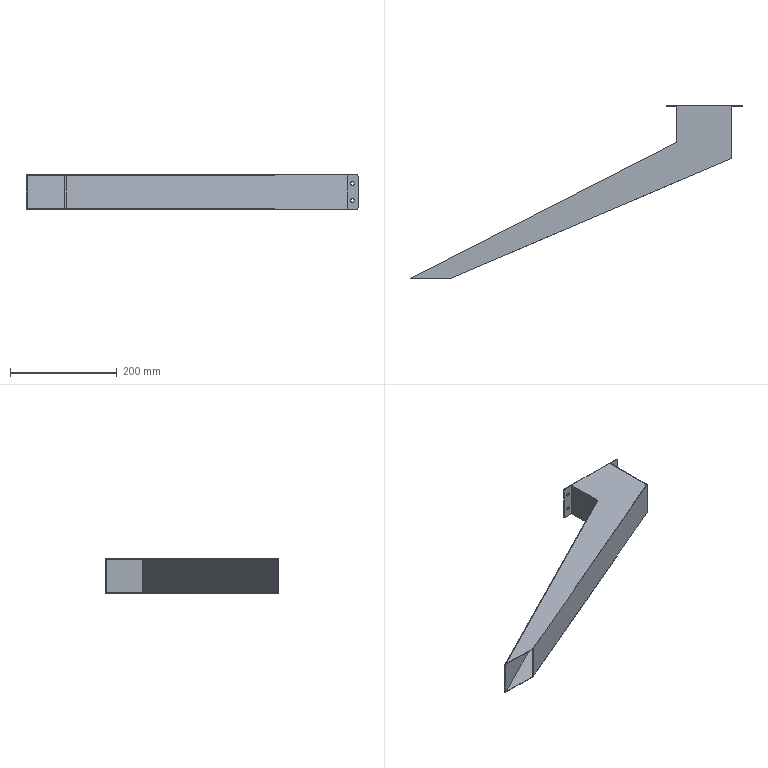Part | NX | 1 solid | 30 faces | box 622 x 324 x 65 mm | volume 159538 mm3 | plane 18 | cylinder 12 | commonest cylinder face diameters 6.4 x8 6 x4
STEP:
#1=CARTESIAN_POINT('',(1439.,-457.5,-79.28));
#2=VERTEX_POINT('',#1);
#3=CARTESIAN_POINT('',(1966.,-232.5,-79.28));
#4=VERTEX_POINT('',#3);
#5=CARTESIAN_POINT('',(1439.,-457.5,-79.28));
#6=DIRECTION('',(0.9197,0.3927,0.));
#7=VECTOR('',#6,1000.);
#8=LINE('',#5,#7);
#9=EDGE_CURVE('',#2,#4,#8,.T.);
#10=ORIENTED_EDGE('',*,*,#9,.F.);
#11=CARTESIAN_POINT('',(1439.,-457.5,-144.28));
#12=VERTEX_POINT('',#11);
#13=CARTESIAN_POINT('',(1439.,-457.5,-79.28));
#14=DIRECTION('',(0.,0.,-1.));
#15=VECTOR('',#14,1000.);
#16=LINE('',#13,#15);
#17=EDGE_CURVE('',#2,#12,#16,.T.);
#18=ORIENTED_EDGE('',*,*,#17,.T.);
#19=CARTESIAN_POINT('',(1966.,-232.5,-144.28));
#20=VERTEX_POINT('',#19);
#21=CARTESIAN_POINT('',(1439.,-457.5,-144.28));
#22=DIRECTION('',(0.9197,0.3927,0.));
#23=VECTOR('',#22,1000.);
#24=LINE('',#21,#23);
#25=EDGE_CURVE('',#12,#20,#24,.T.);
#26=ORIENTED_EDGE('',*,*,#25,.T.);
#27=CARTESIAN_POINT('',(1966.,-232.5,-79.28));
#28=DIRECTION('',(0.,0.,-1.));
#29=VECTOR('',#28,1000.);
#30=LINE('',#27,#29);
#31=EDGE_CURVE('',#4,#20,#30,.T.);
#32=ORIENTED_EDGE('',*,*,#31,.F.);
#33=EDGE_LOOP('',(#10,#18,#26,#32));
#34=FACE_BOUND('',#33,.T.);
#35=CARTESIAN_POINT('',(1439.,-457.5,-79.28));
#36=DIRECTION('',(0.3927,-0.9197,0.));
#37=DIRECTION('',(0.,0.,-1.));
#38=AXIS2_PLACEMENT_3D('',#35,#36,#37);
#39=PLANE('',#38);
#40=ADVANCED_FACE('',(#34),#39,.T.);
#41=CARTESIAN_POINT('',(1364.,-457.5,-79.28));
#42=VERTEX_POINT('',#41);
#43=CARTESIAN_POINT('',(1439.,-457.5,-79.28));
#44=DIRECTION('',(-1.,0.,0.));
#45=VECTOR('',#44,1000.);
#46=LINE('',#43,#45);
#47=EDGE_CURVE('',#2,#42,#46,.T.);
#48=ORIENTED_EDGE('',*,*,#47,.T.);
#49=CARTESIAN_POINT('',(1364.,-457.5,-144.28));
#50=VERTEX_POINT('',#49);
#51=CARTESIAN_POINT('',(1364.,-457.5,-79.28));
#52=DIRECTION('',(0.,0.,-1.));
#53=VECTOR('',#52,1000.);
#54=LINE('',#51,#53);
#55=EDGE_CURVE('',#42,#50,#54,.T.);
#56=ORIENTED_EDGE('',*,*,#55,.T.);
#57=CARTESIAN_POINT('',(1439.,-457.5,-144.28));
#58=DIRECTION('',(-1.,0.,0.));
#59=VECTOR('',#58,1000.);
#60=LINE('',#57,#59);
#61=EDGE_CURVE('',#12,#50,#60,.T.);
#62=ORIENTED_EDGE('',*,*,#61,.F.);
#63=ORIENTED_EDGE('',*,*,#17,.F.);
#64=EDGE_LOOP('',(#48,#56,#62,#63));
#65=FACE_BOUND('',#64,.T.);
#66=CARTESIAN_POINT('',(1436.453,-457.5,-143.28));
#67=VERTEX_POINT('',#66);
#68=CARTESIAN_POINT('',(1436.453,-457.5,-80.28));
#69=VERTEX_POINT('',#68);
#70=CARTESIAN_POINT('',(1436.453,-457.5,-79.28));
#71=DIRECTION('',(0.,0.,1.));
#72=VECTOR('',#71,1000.);
#73=LINE('',#70,#72);
#74=EDGE_CURVE('',#67,#69,#73,.T.);
#75=ORIENTED_EDGE('',*,*,#74,.F.);
#76=CARTESIAN_POINT('',(1366.201,-457.5,-143.28));
#77=VERTEX_POINT('',#76);
#78=CARTESIAN_POINT('',(1903.812,-457.5,-143.28));
#79=DIRECTION('',(-1.,0.,0.));
#80=VECTOR('',#79,1000.);
#81=LINE('',#78,#80);
#82=EDGE_CURVE('',#67,#77,#81,.T.);
#83=ORIENTED_EDGE('',*,*,#82,.T.);
#84=CARTESIAN_POINT('',(1366.201,-457.5,-80.28));
#85=VERTEX_POINT('',#84);
#86=CARTESIAN_POINT('',(1366.201,-457.5,-79.28));
#87=DIRECTION('',(0.,0.,-1.));
#88=VECTOR('',#87,1000.);
#89=LINE('',#86,#88);
#90=EDGE_CURVE('',#85,#77,#89,.T.);
#91=ORIENTED_EDGE('',*,*,#90,.F.);
#92=CARTESIAN_POINT('',(1903.812,-457.5,-80.28));
#93=DIRECTION('',(-1.,0.,0.));
#94=VECTOR('',#93,1000.);
#95=LINE('',#92,#94);
#96=EDGE_CURVE('',#69,#85,#95,.T.);
#97=ORIENTED_EDGE('',*,*,#96,.F.);
#98=EDGE_LOOP('',(#75,#83,#91,#97));
#99=FACE_BOUND('',#98,.T.);
#100=CARTESIAN_POINT('',(1364.,-457.5,-79.28));
#101=DIRECTION('',(0.,-1.,0.));
#102=DIRECTION('',(0.,0.,-1.));
#103=AXIS2_PLACEMENT_3D('',#100,#101,#102);
#104=PLANE('',#103);
#105=ADVANCED_FACE('',(#65,#99),#104,.T.);
#106=CARTESIAN_POINT('',(1864.,-202.5,-79.28));
#107=VERTEX_POINT('',#106);
#108=CARTESIAN_POINT('',(1364.,-457.5,-79.28));
#109=DIRECTION('',(0.8908,0.4543,0.));
#110=VECTOR('',#109,1000.);
#111=LINE('',#108,#110);
#112=EDGE_CURVE('',#42,#107,#111,.T.);
#113=ORIENTED_EDGE('',*,*,#112,.T.);
#114=CARTESIAN_POINT('',(1864.,-202.5,-144.28));
#115=VERTEX_POINT('',#114);
#116=CARTESIAN_POINT('',(1864.,-202.5,-79.28));
#117=DIRECTION('',(0.,0.,-1.));
#118=VECTOR('',#117,1000.);
#119=LINE('',#116,#118);
#120=EDGE_CURVE('',#107,#115,#119,.T.);
#121=ORIENTED_EDGE('',*,*,#120,.T.);
#122=CARTESIAN_POINT('',(1364.,-457.5,-144.28));
#123=DIRECTION('',(0.8908,0.4543,0.));
#124=VECTOR('',#123,1000.);
#125=LINE('',#122,#124);
#126=EDGE_CURVE('',#50,#115,#125,.T.);
#127=ORIENTED_EDGE('',*,*,#126,.F.);
#128=ORIENTED_EDGE('',*,*,#55,.F.);
#129=EDGE_LOOP('',(#113,#121,#127,#128));
#130=FACE_BOUND('',#129,.T.);
#131=CARTESIAN_POINT('',(1864.,-202.5,-79.28));
#132=DIRECTION('',(-0.4543,0.8908,0.));
#133=DIRECTION('',(0.,0.,1.));
#134=AXIS2_PLACEMENT_3D('',#131,#132,#133);
#135=PLANE('',#134);
#136=ADVANCED_FACE('',(#130),#135,.T.);
#137=CARTESIAN_POINT('',(1864.,-134.5,-79.28));
#138=VERTEX_POINT('',#137);
#139=CARTESIAN_POINT('',(1864.,-134.5,-144.28));
#140=VERTEX_POINT('',#139);
#141=CARTESIAN_POINT('',(1864.,-134.5,-79.28));
#142=DIRECTION('',(0.,0.,-1.));
#143=VECTOR('',#142,1000.);
#144=LINE('',#141,#143);
#145=EDGE_CURVE('',#138,#140,#144,.T.);
#146=ORIENTED_EDGE('',*,*,#145,.T.);
#147=CARTESIAN_POINT('',(1864.,-232.5,-144.28));
#148=DIRECTION('',(0.,1.,0.));
#149=VECTOR('',#148,1000.);
#150=LINE('',#147,#149);
#151=EDGE_CURVE('',#115,#140,#150,.T.);
#152=ORIENTED_EDGE('',*,*,#151,.F.);
#153=ORIENTED_EDGE('',*,*,#120,.F.);
#154=CARTESIAN_POINT('',(1864.,-232.5,-79.28));
#155=DIRECTION('',(0.,1.,0.));
#156=VECTOR('',#155,1000.);
#157=LINE('',#154,#156);
#158=EDGE_CURVE('',#107,#138,#157,.T.);
#159=ORIENTED_EDGE('',*,*,#158,.T.);
#160=EDGE_LOOP('',(#146,#152,#153,#159));
#161=FACE_BOUND('',#160,.T.);
#162=CARTESIAN_POINT('',(1864.,-133.5,-79.28));
#163=DIRECTION('',(-1.,0.,0.));
#164=DIRECTION('',(0.,0.,1.));
#165=AXIS2_PLACEMENT_3D('',#162,#163,#164);
#166=PLANE('',#165);
#167=ADVANCED_FACE('',(#161),#166,.T.);
#168=CARTESIAN_POINT('',(1966.,-134.5,-79.28));
#169=VERTEX_POINT('',#168);
#170=CARTESIAN_POINT('',(1966.,-133.5,-79.28));
#171=DIRECTION('',(0.,-1.,0.));
#172=VECTOR('',#171,1000.);
#173=LINE('',#170,#172);
#174=EDGE_CURVE('',#169,#4,#173,.T.);
#175=ORIENTED_EDGE('',*,*,#174,.T.);
#176=ORIENTED_EDGE('',*,*,#31,.T.);
#177=CARTESIAN_POINT('',(1966.,-134.5,-144.28));
#178=VERTEX_POINT('',#177);
#179=CARTESIAN_POINT('',(1966.,-133.5,-144.28));
#180=DIRECTION('',(0.,-1.,0.));
#181=VECTOR('',#180,1000.);
#182=LINE('',#179,#181);
#183=EDGE_CURVE('',#178,#20,#182,.T.);
#184=ORIENTED_EDGE('',*,*,#183,.F.);
#185=CARTESIAN_POINT('',(1966.,-134.5,-79.28));
#186=DIRECTION('',(0.,0.,1.));
#187=VECTOR('',#186,1000.);
#188=LINE('',#185,#187);
#189=EDGE_CURVE('',#178,#169,#188,.T.);
#190=ORIENTED_EDGE('',*,*,#189,.T.);
#191=EDGE_LOOP('',(#175,#176,#184,#190));
#192=FACE_BOUND('',#191,.T.);
#193=CARTESIAN_POINT('',(1966.,-232.5,-79.28));
#194=DIRECTION('',(1.,0.,0.));
#195=DIRECTION('',(0.,1.,0.));
#196=AXIS2_PLACEMENT_3D('',#193,#194,#195);
#197=PLANE('',#196);
#198=ADVANCED_FACE('',(#192),#197,.T.);
#199=CARTESIAN_POINT('',(1965.,-133.5,-80.28));
#200=VERTEX_POINT('',#199);
#201=CARTESIAN_POINT('',(1965.,-231.84,-80.28));
#202=VERTEX_POINT('',#201);
#203=CARTESIAN_POINT('',(1965.,-133.5,-80.28));
#204=DIRECTION('',(0.,-1.,0.));
#205=VECTOR('',#204,1000.);
#206=LINE('',#203,#205);
#207=EDGE_CURVE('',#200,#202,#206,.T.);
#208=ORIENTED_EDGE('',*,*,#207,.T.);
#209=CARTESIAN_POINT('',(1903.812,-257.964,-80.28));
#210=DIRECTION('',(0.9197,0.3927,0.));
#211=VECTOR('',#210,1000.);
#212=LINE('',#209,#211);
#213=EDGE_CURVE('',#69,#202,#212,.T.);
#214=ORIENTED_EDGE('',*,*,#213,.F.);
#215=ORIENTED_EDGE('',*,*,#96,.T.);
#216=CARTESIAN_POINT('',(1865.,-203.113,-80.28));
#217=VERTEX_POINT('',#216);
#218=CARTESIAN_POINT('',(1903.812,-183.319,-80.28));
#219=DIRECTION('',(0.8908,0.4543,0.));
#220=VECTOR('',#219,1000.);
#221=LINE('',#218,#220);
#222=EDGE_CURVE('',#85,#217,#221,.T.);
#223=ORIENTED_EDGE('',*,*,#222,.T.);
#224=CARTESIAN_POINT('',(1865.,-133.5,-80.28));
#225=VERTEX_POINT('',#224);
#226=CARTESIAN_POINT('',(1865.,-24.838,-80.28));
#227=DIRECTION('',(0.,-1.,0.));
#228=VECTOR('',#227,1000.);
#229=LINE('',#226,#228);
#230=EDGE_CURVE('',#225,#217,#229,.T.);
#231=ORIENTED_EDGE('',*,*,#230,.F.);
#232=CARTESIAN_POINT('',(1903.812,-133.5,-80.28));
#233=DIRECTION('',(1.,0.,0.));
#234=VECTOR('',#233,1000.);
#235=LINE('',#232,#234);
#236=EDGE_CURVE('',#225,#200,#235,.T.);
#237=ORIENTED_EDGE('',*,*,#236,.T.);
#238=EDGE_LOOP('',(#208,#214,#215,#223,#231,#237));
#239=FACE_BOUND('',#238,.T.);
#240=CARTESIAN_POINT('',(1903.812,-24.838,-80.28));
#241=DIRECTION('',(0.,0.,1.));
#242=DIRECTION('',(1.,0.,0.));
#243=AXIS2_PLACEMENT_3D('',#240,#241,#242);
#244=PLANE('',#243);
#245=ADVANCED_FACE('',(#239),#244,.F.);
#246=CARTESIAN_POINT('',(1965.,-231.84,-143.28));
#247=VERTEX_POINT('',#246);
#248=CARTESIAN_POINT('',(1965.,-231.84,-79.28));
#249=DIRECTION('',(0.,0.,-1.));
#250=VECTOR('',#249,1000.);
#251=LINE('',#248,#250);
#252=EDGE_CURVE('',#202,#247,#251,.T.);
#253=ORIENTED_EDGE('',*,*,#252,.T.);
#254=CARTESIAN_POINT('',(1903.812,-257.964,-143.28));
#255=DIRECTION('',(0.9197,0.3927,0.));
#256=VECTOR('',#255,1000.);
#257=LINE('',#254,#256);
#258=EDGE_CURVE('',#67,#247,#257,.T.);
#259=ORIENTED_EDGE('',*,*,#258,.F.);
#260=ORIENTED_EDGE('',*,*,#74,.T.);
#261=ORIENTED_EDGE('',*,*,#213,.T.);
#262=EDGE_LOOP('',(#253,#259,#260,#261));
#263=FACE_BOUND('',#262,.T.);
#264=CARTESIAN_POINT('',(1438.607,-456.58,-79.28));
#265=DIRECTION('',(0.3927,-0.9197,0.));
#266=DIRECTION('',(0.,0.,-1.));
#267=AXIS2_PLACEMENT_3D('',#264,#265,#266);
#268=PLANE('',#267);
#269=ADVANCED_FACE('',(#263),#268,.F.);
#270=CARTESIAN_POINT('',(1965.,-133.5,-143.28));
#271=VERTEX_POINT('',#270);
#272=CARTESIAN_POINT('',(1965.,-24.838,-143.28));
#273=DIRECTION('',(0.,-1.,0.));
#274=VECTOR('',#273,1000.);
#275=LINE('',#272,#274);
#276=EDGE_CURVE('',#271,#247,#275,.T.);
#277=ORIENTED_EDGE('',*,*,#276,.T.);
#278=ORIENTED_EDGE('',*,*,#252,.F.);
#279=ORIENTED_EDGE('',*,*,#207,.F.);
#280=CARTESIAN_POINT('',(1965.,-133.5,-79.28));
#281=DIRECTION('',(0.,0.,-1.));
#282=VECTOR('',#281,1000.);
#283=LINE('',#280,#282);
#284=EDGE_CURVE('',#200,#271,#283,.T.);
#285=ORIENTED_EDGE('',*,*,#284,.T.);
#286=EDGE_LOOP('',(#277,#278,#279,#285));
#287=FACE_BOUND('',#286,.T.);
#288=CARTESIAN_POINT('',(1965.,-232.5,-79.28));
#289=DIRECTION('',(1.,0.,0.));
#290=DIRECTION('',(0.,1.,0.));
#291=AXIS2_PLACEMENT_3D('',#288,#289,#290);
#292=PLANE('',#291);
#293=ADVANCED_FACE('',(#287),#292,.F.);
#294=CARTESIAN_POINT('',(1865.,-203.113,-143.28));
#295=VERTEX_POINT('',#294);
#296=CARTESIAN_POINT('',(1865.,-133.5,-143.28));
#297=VERTEX_POINT('',#296);
#298=CARTESIAN_POINT('',(1865.,-24.838,-143.28));
#299=DIRECTION('',(0.,1.,0.));
#300=VECTOR('',#299,1000.);
#301=LINE('',#298,#300);
#302=EDGE_CURVE('',#295,#297,#301,.T.);
#303=ORIENTED_EDGE('',*,*,#302,.F.);
#304=CARTESIAN_POINT('',(1903.812,-183.319,-143.28));
#305=DIRECTION('',(0.8908,0.4543,0.));
#306=VECTOR('',#305,1000.);
#307=LINE('',#304,#306);
#308=EDGE_CURVE('',#77,#295,#307,.T.);
#309=ORIENTED_EDGE('',*,*,#308,.F.);
#310=ORIENTED_EDGE('',*,*,#82,.F.);
#311=ORIENTED_EDGE('',*,*,#258,.T.);
#312=ORIENTED_EDGE('',*,*,#276,.F.);
#313=CARTESIAN_POINT('',(1903.812,-133.5,-143.28));
#314=DIRECTION('',(-1.,0.,0.));
#315=VECTOR('',#314,1000.);
#316=LINE('',#313,#315);
#317=EDGE_CURVE('',#271,#297,#316,.T.);
#318=ORIENTED_EDGE('',*,*,#317,.T.);
#319=EDGE_LOOP('',(#303,#309,#310,#311,#312,#318));
#320=FACE_BOUND('',#319,.T.);
#321=CARTESIAN_POINT('',(1903.812,-24.838,-143.28));
#322=DIRECTION('',(0.,0.,1.));
#323=DIRECTION('',(1.,0.,0.));
#324=AXIS2_PLACEMENT_3D('',#321,#322,#323);
#325=PLANE('',#324);
#326=ADVANCED_FACE('',(#320),#325,.T.);
#327=ORIENTED_EDGE('',*,*,#230,.T.);
#328=CARTESIAN_POINT('',(1865.,-203.113,-79.28));
#329=DIRECTION('',(0.,0.,-1.));
#330=VECTOR('',#329,1000.);
#331=LINE('',#328,#330);
#332=EDGE_CURVE('',#217,#295,#331,.T.);
#333=ORIENTED_EDGE('',*,*,#332,.T.);
#334=ORIENTED_EDGE('',*,*,#302,.T.);
#335=CARTESIAN_POINT('',(1865.,-133.5,-79.28));
#336=DIRECTION('',(0.,0.,1.));
#337=VECTOR('',#336,1000.);
#338=LINE('',#335,#337);
#339=EDGE_CURVE('',#297,#225,#338,.T.);
#340=ORIENTED_EDGE('',*,*,#339,.T.);
#341=EDGE_LOOP('',(#327,#333,#334,#340));
#342=FACE_BOUND('',#341,.T.);
#343=CARTESIAN_POINT('',(1865.,-133.5,-79.28));
#344=DIRECTION('',(-1.,0.,0.));
#345=DIRECTION('',(0.,0.,1.));
#346=AXIS2_PLACEMENT_3D('',#343,#344,#345);
#347=PLANE('',#346);
#348=ADVANCED_FACE('',(#342),#347,.F.);
#349=ORIENTED_EDGE('',*,*,#90,.T.);
#350=ORIENTED_EDGE('',*,*,#308,.T.);
#351=ORIENTED_EDGE('',*,*,#332,.F.);
#352=ORIENTED_EDGE('',*,*,#222,.F.);
#353=EDGE_LOOP('',(#349,#350,#351,#352));
#354=FACE_BOUND('',#353,.T.);
#355=CARTESIAN_POINT('',(1864.454,-203.391,-79.28));
#356=DIRECTION('',(-0.4543,0.8908,0.));
#357=DIRECTION('',(0.,0.,1.));
#358=AXIS2_PLACEMENT_3D('',#355,#356,#357);
#359=PLANE('',#358);
#360=ADVANCED_FACE('',(#354),#359,.F.);
#361=ORIENTED_EDGE('',*,*,#126,.T.);
#362=ORIENTED_EDGE('',*,*,#151,.T.);
#363=CARTESIAN_POINT('',(1847.,-134.5,-144.28));
#364=VERTEX_POINT('',#363);
#365=CARTESIAN_POINT('',(1915.,-134.5,-144.28));
#366=DIRECTION('',(1.,0.,0.));
#367=VECTOR('',#366,1000.);
#368=LINE('',#365,#367);
#369=EDGE_CURVE('',#364,#140,#368,.T.);
#370=ORIENTED_EDGE('',*,*,#369,.F.);
#371=CARTESIAN_POINT('',(1847.,-133.5,-144.28));
#372=VERTEX_POINT('',#371);
#373=CARTESIAN_POINT('',(1847.,-133.5,-144.28));
#374=DIRECTION('',(0.,-1.,0.));
#375=VECTOR('',#374,1000.);
#376=LINE('',#373,#375);
#377=EDGE_CURVE('',#372,#364,#376,.T.);
#378=ORIENTED_EDGE('',*,*,#377,.F.);
#379=CARTESIAN_POINT('',(1983.,-133.5,-144.28));
#380=VERTEX_POINT('',#379);
#381=CARTESIAN_POINT('',(1915.,-133.5,-144.28));
#382=DIRECTION('',(1.,0.,0.));
#383=VECTOR('',#382,1000.);
#384=LINE('',#381,#383);
#385=EDGE_CURVE('',#372,#380,#384,.T.);
#386=ORIENTED_EDGE('',*,*,#385,.T.);
#387=CARTESIAN_POINT('',(1983.,-134.5,-144.28));
#388=VERTEX_POINT('',#387);
#389=CARTESIAN_POINT('',(1983.,-133.5,-144.28));
#390=DIRECTION('',(0.,-1.,0.));
#391=VECTOR('',#390,1000.);
#392=LINE('',#389,#391);
#393=EDGE_CURVE('',#380,#388,#392,.T.);
#394=ORIENTED_EDGE('',*,*,#393,.T.);
#395=CARTESIAN_POINT('',(1915.,-134.5,-144.28));
#396=DIRECTION('',(1.,0.,0.));
#397=VECTOR('',#396,1000.);
#398=LINE('',#395,#397);
#399=EDGE_CURVE('',#178,#388,#398,.T.);
#400=ORIENTED_EDGE('',*,*,#399,.F.);
#401=ORIENTED_EDGE('',*,*,#183,.T.);
#402=ORIENTED_EDGE('',*,*,#25,.F.);
#403=ORIENTED_EDGE('',*,*,#61,.T.);
#404=EDGE_LOOP('',(#361,#362,#370,#378,#386,#394,#400,#401,#402,#403));
#405=FACE_BOUND('',#404,.T.);
#406=CARTESIAN_POINT('',(1903.812,-24.838,-144.28));
#407=DIRECTION('',(0.,0.,1.));
#408=DIRECTION('',(1.,0.,0.));
#409=AXIS2_PLACEMENT_3D('',#406,#407,#408);
#410=PLANE('',#409);
#411=ADVANCED_FACE('',(#405),#410,.F.);
#412=CARTESIAN_POINT('',(1986.,-133.5,-141.28));
#413=VERTEX_POINT('',#412);
#414=CARTESIAN_POINT('',(1983.,-133.5,-141.28));
#415=DIRECTION('',(0.,1.,0.));
#416=DIRECTION('',(1.,0.,0.));
#417=AXIS2_PLACEMENT_3D('',#414,#415,#416);
#418=CIRCLE('',#417,3.);
#419=EDGE_CURVE('',#413,#380,#418,.T.);
#420=ORIENTED_EDGE('',*,*,#419,.F.);
#421=CARTESIAN_POINT('',(1986.,-134.5,-141.28));
#422=VERTEX_POINT('',#421);
#423=CARTESIAN_POINT('',(1986.,-133.5,-141.28));
#424=DIRECTION('',(0.,-1.,0.));
#425=VECTOR('',#424,1000.);
#426=LINE('',#423,#425);
#427=EDGE_CURVE('',#413,#422,#426,.T.);
#428=ORIENTED_EDGE('',*,*,#427,.T.);
#429=CARTESIAN_POINT('',(1983.,-134.5,-141.28));
#430=DIRECTION('',(0.,1.,0.));
#431=DIRECTION('',(1.,0.,0.));
#432=AXIS2_PLACEMENT_3D('',#429,#430,#431);
#433=CIRCLE('',#432,3.);
#434=EDGE_CURVE('',#422,#388,#433,.T.);
#435=ORIENTED_EDGE('',*,*,#434,.T.);
#436=ORIENTED_EDGE('',*,*,#393,.F.);
#437=EDGE_LOOP('',(#420,#428,#435,#436));
#438=FACE_BOUND('',#437,.T.);
#439=CARTESIAN_POINT('',(1983.,-133.5,-141.28));
#440=DIRECTION('',(0.,1.,0.));
#441=DIRECTION('',(1.,0.,0.));
#442=AXIS2_PLACEMENT_3D('',#439,#440,#441);
#443=CYLINDRICAL_SURFACE('',#442,3.);
#444=ADVANCED_FACE('',(#438),#443,.T.);
#445=CARTESIAN_POINT('',(1978.7,-134.5,-127.53));
#446=VERTEX_POINT('',#445);
#447=CARTESIAN_POINT('',(1972.3,-134.5,-127.53));
#448=VERTEX_POINT('',#447);
#449=CARTESIAN_POINT('',(1975.5,-134.5,-127.53));
#450=DIRECTION('',(0.,-1.,0.));
#451=DIRECTION('',(-1.,0.,0.));
#452=AXIS2_PLACEMENT_3D('',#449,#450,#451);
#453=CIRCLE('',#452,3.2);
#454=EDGE_CURVE('',#446,#448,#453,.T.);
#455=ORIENTED_EDGE('',*,*,#454,.T.);
#456=CARTESIAN_POINT('',(1972.3,-133.5,-127.53));
#457=VERTEX_POINT('',#456);
#458=CARTESIAN_POINT('',(1972.3,-133.5,-127.53));
#459=DIRECTION('',(0.,-1.,0.));
#460=VECTOR('',#459,1000.);
#461=LINE('',#458,#460);
#462=EDGE_CURVE('',#448,#457,#461,.F.);
#463=ORIENTED_EDGE('',*,*,#462,.T.);
#464=CARTESIAN_POINT('',(1978.7,-133.5,-127.53));
#465=VERTEX_POINT('',#464);
#466=CARTESIAN_POINT('',(1975.5,-133.5,-127.53));
#467=DIRECTION('',(0.,-1.,0.));
#468=DIRECTION('',(-1.,0.,0.));
#469=AXIS2_PLACEMENT_3D('',#466,#467,#468);
#470=CIRCLE('',#469,3.2);
#471=EDGE_CURVE('',#465,#457,#470,.T.);
#472=ORIENTED_EDGE('',*,*,#471,.F.);
#473=CARTESIAN_POINT('',(1978.7,-133.5,-127.53));
#474=DIRECTION('',(0.,-1.,0.));
#475=VECTOR('',#474,1000.);
#476=LINE('',#473,#475);
#477=EDGE_CURVE('',#446,#465,#476,.F.);
#478=ORIENTED_EDGE('',*,*,#477,.F.);
#479=EDGE_LOOP('',(#455,#463,#472,#478));
#480=FACE_BOUND('',#479,.T.);
#481=CARTESIAN_POINT('',(1975.5,-133.5,-127.53));
#482=DIRECTION('',(0.,-1.,0.));
#483=DIRECTION('',(-1.,0.,0.));
#484=AXIS2_PLACEMENT_3D('',#481,#482,#483);
#485=CYLINDRICAL_SURFACE('',#484,3.2);
#486=ADVANCED_FACE('',(#480),#485,.F.);
#487=CARTESIAN_POINT('',(1978.7,-134.5,-96.03));
#488=VERTEX_POINT('',#487);
#489=CARTESIAN_POINT('',(1972.3,-134.5,-96.03));
#490=VERTEX_POINT('',#489);
#491=CARTESIAN_POINT('',(1975.5,-134.5,-96.03));
#492=DIRECTION('',(0.,-1.,0.));
#493=DIRECTION('',(-1.,0.,0.));
#494=AXIS2_PLACEMENT_3D('',#491,#492,#493);
#495=CIRCLE('',#494,3.2);
#496=EDGE_CURVE('',#488,#490,#495,.T.);
#497=ORIENTED_EDGE('',*,*,#496,.T.);
#498=CARTESIAN_POINT('',(1972.3,-133.5,-96.03));
#499=VERTEX_POINT('',#498);
#500=CARTESIAN_POINT('',(1972.3,-133.5,-96.03));
#501=DIRECTION('',(0.,-1.,0.));
#502=VECTOR('',#501,1000.);
#503=LINE('',#500,#502);
#504=EDGE_CURVE('',#490,#499,#503,.F.);
#505=ORIENTED_EDGE('',*,*,#504,.T.);
#506=CARTESIAN_POINT('',(1978.7,-133.5,-96.03));
#507=VERTEX_POINT('',#506);
#508=CARTESIAN_POINT('',(1975.5,-133.5,-96.03));
#509=DIRECTION('',(0.,-1.,0.));
#510=DIRECTION('',(-1.,0.,0.));
#511=AXIS2_PLACEMENT_3D('',#508,#509,#510);
#512=CIRCLE('',#511,3.2);
#513=EDGE_CURVE('',#507,#499,#512,.T.);
#514=ORIENTED_EDGE('',*,*,#513,.F.);
#515=CARTESIAN_POINT('',(1978.7,-133.5,-96.03));
#516=DIRECTION('',(0.,-1.,0.));
#517=VECTOR('',#516,1000.);
#518=LINE('',#515,#517);
#519=EDGE_CURVE('',#488,#507,#518,.F.);
#520=ORIENTED_EDGE('',*,*,#519,.F.);
#521=EDGE_LOOP('',(#497,#505,#514,#520));
#522=FACE_BOUND('',#521,.T.);
#523=CARTESIAN_POINT('',(1975.5,-133.5,-96.03));
#524=DIRECTION('',(0.,-1.,0.));
#525=DIRECTION('',(-1.,0.,0.));
#526=AXIS2_PLACEMENT_3D('',#523,#524,#525);
#527=CYLINDRICAL_SURFACE('',#526,3.2);
#528=ADVANCED_FACE('',(#522),#527,.F.);
#529=ORIENTED_EDGE('',*,*,#399,.T.);
#530=ORIENTED_EDGE('',*,*,#434,.F.);
#531=CARTESIAN_POINT('',(1986.,-134.5,-82.28));
#532=VERTEX_POINT('',#531);
#533=CARTESIAN_POINT('',(1986.,-134.5,-130.28));
#534=DIRECTION('',(0.,0.,-1.));
#535=VECTOR('',#534,1000.);
#536=LINE('',#533,#535);
#537=EDGE_CURVE('',#532,#422,#536,.T.);
#538=ORIENTED_EDGE('',*,*,#537,.F.);
#539=CARTESIAN_POINT('',(1983.,-134.5,-79.28));
#540=VERTEX_POINT('',#539);
#541=CARTESIAN_POINT('',(1983.,-134.5,-82.28));
#542=DIRECTION('',(0.,1.,0.));
#543=DIRECTION('',(1.,0.,0.));
#544=AXIS2_PLACEMENT_3D('',#541,#542,#543);
#545=CIRCLE('',#544,3.);
#546=EDGE_CURVE('',#540,#532,#545,.T.);
#547=ORIENTED_EDGE('',*,*,#546,.F.);
#548=CARTESIAN_POINT('',(1915.,-134.5,-79.28));
#549=DIRECTION('',(1.,0.,0.));
#550=VECTOR('',#549,1000.);
#551=LINE('',#548,#550);
#552=EDGE_CURVE('',#169,#540,#551,.T.);
#553=ORIENTED_EDGE('',*,*,#552,.F.);
#554=ORIENTED_EDGE('',*,*,#189,.F.);
#555=EDGE_LOOP('',(#529,#530,#538,#547,#553,#554));
#556=FACE_BOUND('',#555,.T.);
#557=ORIENTED_EDGE('',*,*,#454,.F.);
#558=CARTESIAN_POINT('',(1975.5,-134.5,-127.53));
#559=DIRECTION('',(0.,-1.,0.));
#560=DIRECTION('',(-1.,0.,0.));
#561=AXIS2_PLACEMENT_3D('',#558,#559,#560);
#562=CIRCLE('',#561,3.2);
#563=EDGE_CURVE('',#448,#446,#562,.T.);
#564=ORIENTED_EDGE('',*,*,#563,.F.);
#565=EDGE_LOOP('',(#557,#564));
#566=FACE_BOUND('',#565,.T.);
#567=ORIENTED_EDGE('',*,*,#496,.F.);
#568=CARTESIAN_POINT('',(1975.5,-134.5,-96.03));
#569=DIRECTION('',(0.,-1.,0.));
#570=DIRECTION('',(-1.,0.,0.));
#571=AXIS2_PLACEMENT_3D('',#568,#569,#570);
#572=CIRCLE('',#571,3.2);
#573=EDGE_CURVE('',#490,#488,#572,.T.);
#574=ORIENTED_EDGE('',*,*,#573,.F.);
#575=EDGE_LOOP('',(#567,#574));
#576=FACE_BOUND('',#575,.T.);
#577=CARTESIAN_POINT('',(1876.658,-134.5,-112.212));
#578=DIRECTION('',(0.,1.,0.));
#579=DIRECTION('',(1.,0.,0.));
#580=AXIS2_PLACEMENT_3D('',#577,#578,#579);
#581=PLANE('',#580);
#582=ADVANCED_FACE('',(#556,#566,#576),#581,.F.);
#583=CARTESIAN_POINT('',(1983.,-133.5,-79.28));
#584=VERTEX_POINT('',#583);
#585=CARTESIAN_POINT('',(1986.,-133.5,-82.28));
#586=VERTEX_POINT('',#585);
#587=CARTESIAN_POINT('',(1983.,-133.5,-82.28));
#588=DIRECTION('',(0.,1.,0.));
#589=DIRECTION('',(1.,0.,0.));
#590=AXIS2_PLACEMENT_3D('',#587,#588,#589);
#591=CIRCLE('',#590,3.);
#592=EDGE_CURVE('',#584,#586,#591,.T.);
#593=ORIENTED_EDGE('',*,*,#592,.F.);
#594=CARTESIAN_POINT('',(1983.,-133.5,-79.28));
#595=DIRECTION('',(0.,-1.,0.));
#596=VECTOR('',#595,1000.);
#597=LINE('',#594,#596);
#598=EDGE_CURVE('',#584,#540,#597,.T.);
#599=ORIENTED_EDGE('',*,*,#598,.T.);
#600=ORIENTED_EDGE('',*,*,#546,.T.);
#601=CARTESIAN_POINT('',(1986.,-133.5,-82.28));
#602=DIRECTION('',(0.,-1.,0.));
#603=VECTOR('',#602,1000.);
#604=LINE('',#601,#603);
#605=EDGE_CURVE('',#586,#532,#604,.T.);
#606=ORIENTED_EDGE('',*,*,#605,.F.);
#607=EDGE_LOOP('',(#593,#599,#600,#606));
#608=FACE_BOUND('',#607,.T.);
#609=CARTESIAN_POINT('',(1983.,-133.5,-82.28));
#610=DIRECTION('',(0.,1.,0.));
#611=DIRECTION('',(1.,0.,0.));
#612=AXIS2_PLACEMENT_3D('',#609,#610,#611);
#613=CYLINDRICAL_SURFACE('',#612,3.);
#614=ADVANCED_FACE('',(#608),#613,.T.);
#615=CARTESIAN_POINT('',(1986.,-133.5,-130.28));
#616=DIRECTION('',(0.,0.,-1.));
#617=VECTOR('',#616,1000.);
#618=LINE('',#615,#617);
#619=EDGE_CURVE('',#586,#413,#618,.T.);
#620=ORIENTED_EDGE('',*,*,#619,.F.);
#621=ORIENTED_EDGE('',*,*,#605,.T.);
#622=ORIENTED_EDGE('',*,*,#537,.T.);
#623=ORIENTED_EDGE('',*,*,#427,.F.);
#624=EDGE_LOOP('',(#620,#621,#622,#623));
#625=FACE_BOUND('',#624,.T.);
#626=CARTESIAN_POINT('',(1986.,-133.5,-82.28));
#627=DIRECTION('',(1.,0.,0.));
#628=DIRECTION('',(0.,1.,0.));
#629=AXIS2_PLACEMENT_3D('',#626,#627,#628);
#630=PLANE('',#629);
#631=ADVANCED_FACE('',(#625),#630,.T.);
#632=ORIENTED_EDGE('',*,*,#462,.F.);
#633=ORIENTED_EDGE('',*,*,#563,.T.);
#634=ORIENTED_EDGE('',*,*,#477,.T.);
#635=CARTESIAN_POINT('',(1975.5,-133.5,-127.53));
#636=DIRECTION('',(0.,-1.,0.));
#637=DIRECTION('',(-1.,0.,0.));
#638=AXIS2_PLACEMENT_3D('',#635,#636,#637);
#639=CIRCLE('',#638,3.2);
#640=EDGE_CURVE('',#457,#465,#639,.T.);
#641=ORIENTED_EDGE('',*,*,#640,.F.);
#642=EDGE_LOOP('',(#632,#633,#634,#641));
#643=FACE_BOUND('',#642,.T.);
#644=CARTESIAN_POINT('',(1975.5,-133.5,-127.53));
#645=DIRECTION('',(0.,-1.,0.));
#646=DIRECTION('',(-1.,0.,0.));
#647=AXIS2_PLACEMENT_3D('',#644,#645,#646);
#648=CYLINDRICAL_SURFACE('',#647,3.2);
#649=ADVANCED_FACE('',(#643),#648,.F.);
#650=ORIENTED_EDGE('',*,*,#504,.F.);
#651=ORIENTED_EDGE('',*,*,#573,.T.);
#652=ORIENTED_EDGE('',*,*,#519,.T.);
#653=CARTESIAN_POINT('',(1975.5,-133.5,-96.03));
#654=DIRECTION('',(0.,-1.,0.));
#655=DIRECTION('',(-1.,0.,0.));
#656=AXIS2_PLACEMENT_3D('',#653,#654,#655);
#657=CIRCLE('',#656,3.2);
#658=EDGE_CURVE('',#499,#507,#657,.T.);
#659=ORIENTED_EDGE('',*,*,#658,.F.);
#660=EDGE_LOOP('',(#650,#651,#652,#659));
#661=FACE_BOUND('',#660,.T.);
#662=CARTESIAN_POINT('',(1975.5,-133.5,-96.03));
#663=DIRECTION('',(0.,-1.,0.));
#664=DIRECTION('',(-1.,0.,0.));
#665=AXIS2_PLACEMENT_3D('',#662,#663,#664);
#666=CYLINDRICAL_SURFACE('',#665,3.2);
#667=ADVANCED_FACE('',(#661),#666,.F.);
#668=CARTESIAN_POINT('',(1857.7,-134.5,-96.03));
#669=VERTEX_POINT('',#668);
#670=CARTESIAN_POINT('',(1851.3,-134.5,-96.03));
#671=VERTEX_POINT('',#670);
#672=CARTESIAN_POINT('',(1854.5,-134.5,-96.03));
#673=DIRECTION('',(0.,-1.,0.));
#674=DIRECTION('',(-1.,0.,0.));
#675=AXIS2_PLACEMENT_3D('',#672,#673,#674);
#676=CIRCLE('',#675,3.2);
#677=EDGE_CURVE('',#669,#671,#676,.T.);
#678=ORIENTED_EDGE('',*,*,#677,.T.);
#679=CARTESIAN_POINT('',(1851.3,-133.5,-96.03));
#680=VERTEX_POINT('',#679);
#681=CARTESIAN_POINT('',(1851.3,-133.5,-96.03));
#682=DIRECTION('',(0.,-1.,0.));
#683=VECTOR('',#682,1000.);
#684=LINE('',#681,#683);
#685=EDGE_CURVE('',#671,#680,#684,.F.);
#686=ORIENTED_EDGE('',*,*,#685,.T.);
#687=CARTESIAN_POINT('',(1857.7,-133.5,-96.03));
#688=VERTEX_POINT('',#687);
#689=CARTESIAN_POINT('',(1854.5,-133.5,-96.03));
#690=DIRECTION('',(0.,-1.,0.));
#691=DIRECTION('',(-1.,0.,0.));
#692=AXIS2_PLACEMENT_3D('',#689,#690,#691);
#693=CIRCLE('',#692,3.2);
#694=EDGE_CURVE('',#688,#680,#693,.T.);
#695=ORIENTED_EDGE('',*,*,#694,.F.);
#696=CARTESIAN_POINT('',(1857.7,-133.5,-96.03));
#697=DIRECTION('',(0.,-1.,0.));
#698=VECTOR('',#697,1000.);
#699=LINE('',#696,#698);
#700=EDGE_CURVE('',#669,#688,#699,.F.);
#701=ORIENTED_EDGE('',*,*,#700,.F.);
#702=EDGE_LOOP('',(#678,#686,#695,#701));
#703=FACE_BOUND('',#702,.T.);
#704=CARTESIAN_POINT('',(1854.5,-133.5,-96.03));
#705=DIRECTION('',(0.,-1.,0.));
#706=DIRECTION('',(-1.,0.,0.));
#707=AXIS2_PLACEMENT_3D('',#704,#705,#706);
#708=CYLINDRICAL_SURFACE('',#707,3.2);
#709=ADVANCED_FACE('',(#703),#708,.F.);
#710=ORIENTED_EDGE('',*,*,#552,.T.);
#711=ORIENTED_EDGE('',*,*,#598,.F.);
#712=CARTESIAN_POINT('',(1847.,-133.5,-79.28));
#713=VERTEX_POINT('',#712);
#714=CARTESIAN_POINT('',(1915.,-133.5,-79.28));
#715=DIRECTION('',(1.,0.,0.));
#716=VECTOR('',#715,1000.);
#717=LINE('',#714,#716);
#718=EDGE_CURVE('',#713,#584,#717,.T.);
#719=ORIENTED_EDGE('',*,*,#718,.F.);
#720=CARTESIAN_POINT('',(1847.,-134.5,-79.28));
#721=VERTEX_POINT('',#720);
#722=CARTESIAN_POINT('',(1847.,-133.5,-79.28));
#723=DIRECTION('',(0.,-1.,0.));
#724=VECTOR('',#723,1000.);
#725=LINE('',#722,#724);
#726=EDGE_CURVE('',#713,#721,#725,.T.);
#727=ORIENTED_EDGE('',*,*,#726,.T.);
#728=CARTESIAN_POINT('',(1915.,-134.5,-79.28));
#729=DIRECTION('',(1.,0.,0.));
#730=VECTOR('',#729,1000.);
#731=LINE('',#728,#730);
#732=EDGE_CURVE('',#721,#138,#731,.T.);
#733=ORIENTED_EDGE('',*,*,#732,.T.);
#734=ORIENTED_EDGE('',*,*,#158,.F.);
#735=ORIENTED_EDGE('',*,*,#112,.F.);
#736=ORIENTED_EDGE('',*,*,#47,.F.);
#737=ORIENTED_EDGE('',*,*,#9,.T.);
#738=ORIENTED_EDGE('',*,*,#174,.F.);
#739=EDGE_LOOP('',(#710,#711,#719,#727,#733,#734,#735,#736,#737,#738));
#740=FACE_BOUND('',#739,.T.);
#741=CARTESIAN_POINT('',(1903.812,-24.838,-79.28));
#742=DIRECTION('',(0.,0.,1.));
#743=DIRECTION('',(1.,0.,0.));
#744=AXIS2_PLACEMENT_3D('',#741,#742,#743);
#745=PLANE('',#744);
#746=ADVANCED_FACE('',(#740),#745,.T.);
#747=CARTESIAN_POINT('',(1844.,-133.5,-82.28));
#748=VERTEX_POINT('',#747);
#749=CARTESIAN_POINT('',(1847.,-133.5,-82.28));
#750=DIRECTION('',(0.,-1.,0.));
#751=DIRECTION('',(-1.,0.,0.));
#752=AXIS2_PLACEMENT_3D('',#749,#750,#751);
#753=CIRCLE('',#752,3.);
#754=EDGE_CURVE('',#713,#748,#753,.T.);
#755=ORIENTED_EDGE('',*,*,#754,.T.);
#756=CARTESIAN_POINT('',(1844.,-134.5,-82.28));
#757=VERTEX_POINT('',#756);
#758=CARTESIAN_POINT('',(1844.,-133.5,-82.28));
#759=DIRECTION('',(0.,-1.,0.));
#760=VECTOR('',#759,1000.);
#761=LINE('',#758,#760);
#762=EDGE_CURVE('',#748,#757,#761,.T.);
#763=ORIENTED_EDGE('',*,*,#762,.T.);
#764=CARTESIAN_POINT('',(1847.,-134.5,-82.28));
#765=DIRECTION('',(0.,-1.,0.));
#766=DIRECTION('',(-1.,0.,0.));
#767=AXIS2_PLACEMENT_3D('',#764,#765,#766);
#768=CIRCLE('',#767,3.);
#769=EDGE_CURVE('',#721,#757,#768,.T.);
#770=ORIENTED_EDGE('',*,*,#769,.F.);
#771=ORIENTED_EDGE('',*,*,#726,.F.);
#772=EDGE_LOOP('',(#755,#763,#770,#771));
#773=FACE_BOUND('',#772,.T.);
#774=CARTESIAN_POINT('',(1847.,-133.5,-82.28));
#775=DIRECTION('',(0.,-1.,0.));
#776=DIRECTION('',(-1.,0.,0.));
#777=AXIS2_PLACEMENT_3D('',#774,#775,#776);
#778=CYLINDRICAL_SURFACE('',#777,3.);
#779=ADVANCED_FACE('',(#773),#778,.T.);
#780=CARTESIAN_POINT('',(1844.,-133.5,-141.28));
#781=VERTEX_POINT('',#780);
#782=CARTESIAN_POINT('',(1844.,-133.5,-130.28));
#783=DIRECTION('',(0.,0.,1.));
#784=VECTOR('',#783,1000.);
#785=LINE('',#782,#784);
#786=EDGE_CURVE('',#781,#748,#785,.T.);
#787=ORIENTED_EDGE('',*,*,#786,.F.);
#788=CARTESIAN_POINT('',(1844.,-134.5,-141.28));
#789=VERTEX_POINT('',#788);
#790=CARTESIAN_POINT('',(1844.,-133.5,-141.28));
#791=DIRECTION('',(0.,-1.,0.));
#792=VECTOR('',#791,1000.);
#793=LINE('',#790,#792);
#794=EDGE_CURVE('',#781,#789,#793,.T.);
#795=ORIENTED_EDGE('',*,*,#794,.T.);
#796=CARTESIAN_POINT('',(1844.,-134.5,-130.28));
#797=DIRECTION('',(0.,0.,1.));
#798=VECTOR('',#797,1000.);
#799=LINE('',#796,#798);
#800=EDGE_CURVE('',#789,#757,#799,.T.);
#801=ORIENTED_EDGE('',*,*,#800,.T.);
#802=ORIENTED_EDGE('',*,*,#762,.F.);
#803=EDGE_LOOP('',(#787,#795,#801,#802));
#804=FACE_BOUND('',#803,.T.);
#805=CARTESIAN_POINT('',(1844.,-133.5,-141.28));
#806=DIRECTION('',(-1.,0.,0.));
#807=DIRECTION('',(0.,0.,1.));
#808=AXIS2_PLACEMENT_3D('',#805,#806,#807);
#809=PLANE('',#808);
#810=ADVANCED_FACE('',(#804),#809,.T.);
#811=CARTESIAN_POINT('',(1847.,-133.5,-141.28));
#812=DIRECTION('',(0.,-1.,0.));
#813=DIRECTION('',(-1.,0.,0.));
#814=AXIS2_PLACEMENT_3D('',#811,#812,#813);
#815=CIRCLE('',#814,3.);
#816=EDGE_CURVE('',#781,#372,#815,.T.);
#817=ORIENTED_EDGE('',*,*,#816,.T.);
#818=ORIENTED_EDGE('',*,*,#377,.T.);
#819=CARTESIAN_POINT('',(1847.,-134.5,-141.28));
#820=DIRECTION('',(0.,-1.,0.));
#821=DIRECTION('',(-1.,0.,0.));
#822=AXIS2_PLACEMENT_3D('',#819,#820,#821);
#823=CIRCLE('',#822,3.);
#824=EDGE_CURVE('',#789,#364,#823,.T.);
#825=ORIENTED_EDGE('',*,*,#824,.F.);
#826=ORIENTED_EDGE('',*,*,#794,.F.);
#827=EDGE_LOOP('',(#817,#818,#825,#826));
#828=FACE_BOUND('',#827,.T.);
#829=CARTESIAN_POINT('',(1847.,-133.5,-141.28));
#830=DIRECTION('',(0.,-1.,0.));
#831=DIRECTION('',(-1.,0.,0.));
#832=AXIS2_PLACEMENT_3D('',#829,#830,#831);
#833=CYLINDRICAL_SURFACE('',#832,3.);
#834=ADVANCED_FACE('',(#828),#833,.T.);
#835=ORIENTED_EDGE('',*,*,#145,.F.);
#836=ORIENTED_EDGE('',*,*,#732,.F.);
#837=ORIENTED_EDGE('',*,*,#769,.T.);
#838=ORIENTED_EDGE('',*,*,#800,.F.);
#839=ORIENTED_EDGE('',*,*,#824,.T.);
#840=ORIENTED_EDGE('',*,*,#369,.T.);
#841=EDGE_LOOP('',(#835,#836,#837,#838,#839,#840));
#842=FACE_BOUND('',#841,.T.);
#843=CARTESIAN_POINT('',(1857.7,-134.5,-127.53));
#844=VERTEX_POINT('',#843);
#845=CARTESIAN_POINT('',(1851.3,-134.5,-127.53));
#846=VERTEX_POINT('',#845);
#847=CARTESIAN_POINT('',(1854.5,-134.5,-127.53));
#848=DIRECTION('',(0.,-1.,0.));
#849=DIRECTION('',(-1.,0.,0.));
#850=AXIS2_PLACEMENT_3D('',#847,#848,#849);
#851=CIRCLE('',#850,3.2);
#852=EDGE_CURVE('',#844,#846,#851,.T.);
#853=ORIENTED_EDGE('',*,*,#852,.F.);
#854=CARTESIAN_POINT('',(1854.5,-134.5,-127.53));
#855=DIRECTION('',(0.,-1.,0.));
#856=DIRECTION('',(-1.,0.,0.));
#857=AXIS2_PLACEMENT_3D('',#854,#855,#856);
#858=CIRCLE('',#857,3.2);
#859=EDGE_CURVE('',#846,#844,#858,.T.);
#860=ORIENTED_EDGE('',*,*,#859,.F.);
#861=EDGE_LOOP('',(#853,#860));
#862=FACE_BOUND('',#861,.T.);
#863=ORIENTED_EDGE('',*,*,#677,.F.);
#864=CARTESIAN_POINT('',(1854.5,-134.5,-96.03));
#865=DIRECTION('',(0.,-1.,0.));
#866=DIRECTION('',(-1.,0.,0.));
#867=AXIS2_PLACEMENT_3D('',#864,#865,#866);
#868=CIRCLE('',#867,3.2);
#869=EDGE_CURVE('',#671,#669,#868,.T.);
#870=ORIENTED_EDGE('',*,*,#869,.F.);
#871=EDGE_LOOP('',(#863,#870));
#872=FACE_BOUND('',#871,.T.);
#873=CARTESIAN_POINT('',(1876.658,-134.5,-112.212));
#874=DIRECTION('',(0.,1.,0.));
#875=DIRECTION('',(1.,0.,0.));
#876=AXIS2_PLACEMENT_3D('',#873,#874,#875);
#877=PLANE('',#876);
#878=ADVANCED_FACE('',(#842,#862,#872),#877,.F.);
#879=ORIENTED_EDGE('',*,*,#852,.T.);
#880=CARTESIAN_POINT('',(1851.3,-133.5,-127.53));
#881=VERTEX_POINT('',#880);
#882=CARTESIAN_POINT('',(1851.3,-133.5,-127.53));
#883=DIRECTION('',(0.,-1.,0.));
#884=VECTOR('',#883,1000.);
#885=LINE('',#882,#884);
#886=EDGE_CURVE('',#846,#881,#885,.F.);
#887=ORIENTED_EDGE('',*,*,#886,.T.);
#888=CARTESIAN_POINT('',(1857.7,-133.5,-127.53));
#889=VERTEX_POINT('',#888);
#890=CARTESIAN_POINT('',(1854.5,-133.5,-127.53));
#891=DIRECTION('',(0.,-1.,0.));
#892=DIRECTION('',(-1.,0.,0.));
#893=AXIS2_PLACEMENT_3D('',#890,#891,#892);
#894=CIRCLE('',#893,3.2);
#895=EDGE_CURVE('',#889,#881,#894,.T.);
#896=ORIENTED_EDGE('',*,*,#895,.F.);
#897=CARTESIAN_POINT('',(1857.7,-133.5,-127.53));
#898=DIRECTION('',(0.,-1.,0.));
#899=VECTOR('',#898,1000.);
#900=LINE('',#897,#899);
#901=EDGE_CURVE('',#844,#889,#900,.F.);
#902=ORIENTED_EDGE('',*,*,#901,.F.);
#903=EDGE_LOOP('',(#879,#887,#896,#902));
#904=FACE_BOUND('',#903,.T.);
#905=CARTESIAN_POINT('',(1854.5,-133.5,-127.53));
#906=DIRECTION('',(0.,-1.,0.));
#907=DIRECTION('',(-1.,0.,0.));
#908=AXIS2_PLACEMENT_3D('',#905,#906,#907);
#909=CYLINDRICAL_SURFACE('',#908,3.2);
#910=ADVANCED_FACE('',(#904),#909,.F.);
#911=ORIENTED_EDGE('',*,*,#816,.F.);
#912=ORIENTED_EDGE('',*,*,#786,.T.);
#913=ORIENTED_EDGE('',*,*,#754,.F.);
#914=ORIENTED_EDGE('',*,*,#718,.T.);
#915=ORIENTED_EDGE('',*,*,#592,.T.);
#916=ORIENTED_EDGE('',*,*,#619,.T.);
#917=ORIENTED_EDGE('',*,*,#419,.T.);
#918=ORIENTED_EDGE('',*,*,#385,.F.);
#919=EDGE_LOOP('',(#911,#912,#913,#914,#915,#916,#917,#918));
#920=FACE_BOUND('',#919,.T.);
#921=ORIENTED_EDGE('',*,*,#895,.T.);
#922=CARTESIAN_POINT('',(1854.5,-133.5,-127.53));
#923=DIRECTION('',(0.,-1.,0.));
#924=DIRECTION('',(-1.,0.,0.));
#925=AXIS2_PLACEMENT_3D('',#922,#923,#924);
#926=CIRCLE('',#925,3.2);
#927=EDGE_CURVE('',#881,#889,#926,.T.);
#928=ORIENTED_EDGE('',*,*,#927,.T.);
#929=EDGE_LOOP('',(#921,#928));
#930=FACE_BOUND('',#929,.T.);
#931=ORIENTED_EDGE('',*,*,#694,.T.);
#932=CARTESIAN_POINT('',(1854.5,-133.5,-96.03));
#933=DIRECTION('',(0.,-1.,0.));
#934=DIRECTION('',(-1.,0.,0.));
#935=AXIS2_PLACEMENT_3D('',#932,#933,#934);
#936=CIRCLE('',#935,3.2);
#937=EDGE_CURVE('',#680,#688,#936,.T.);
#938=ORIENTED_EDGE('',*,*,#937,.T.);
#939=EDGE_LOOP('',(#931,#938));
#940=FACE_BOUND('',#939,.T.);
#941=ORIENTED_EDGE('',*,*,#471,.T.);
#942=ORIENTED_EDGE('',*,*,#640,.T.);
#943=EDGE_LOOP('',(#941,#942));
#944=FACE_BOUND('',#943,.T.);
#945=ORIENTED_EDGE('',*,*,#513,.T.);
#946=ORIENTED_EDGE('',*,*,#658,.T.);
#947=EDGE_LOOP('',(#945,#946));
#948=FACE_BOUND('',#947,.T.);
#949=ORIENTED_EDGE('',*,*,#236,.F.);
#950=ORIENTED_EDGE('',*,*,#339,.F.);
#951=ORIENTED_EDGE('',*,*,#317,.F.);
#952=ORIENTED_EDGE('',*,*,#284,.F.);
#953=EDGE_LOOP('',(#949,#950,#951,#952));
#954=FACE_BOUND('',#953,.T.);
#955=CARTESIAN_POINT('',(1876.658,-133.5,-112.212));
#956=DIRECTION('',(0.,1.,0.));
#957=DIRECTION('',(1.,0.,0.));
#958=AXIS2_PLACEMENT_3D('',#955,#956,#957);
#959=PLANE('',#958);
#960=ADVANCED_FACE('',(#920,#930,#940,#944,#948,#954),#959,.T.);
#961=ORIENTED_EDGE('',*,*,#685,.F.);
#962=ORIENTED_EDGE('',*,*,#869,.T.);
#963=ORIENTED_EDGE('',*,*,#700,.T.);
#964=ORIENTED_EDGE('',*,*,#937,.F.);
#965=EDGE_LOOP('',(#961,#962,#963,#964));
#966=FACE_BOUND('',#965,.T.);
#967=CARTESIAN_POINT('',(1854.5,-133.5,-96.03));
#968=DIRECTION('',(0.,-1.,0.));
#969=DIRECTION('',(-1.,0.,0.));
#970=AXIS2_PLACEMENT_3D('',#967,#968,#969);
#971=CYLINDRICAL_SURFACE('',#970,3.2);
#972=ADVANCED_FACE('',(#966),#971,.F.);
#973=ORIENTED_EDGE('',*,*,#886,.F.);
#974=ORIENTED_EDGE('',*,*,#859,.T.);
#975=ORIENTED_EDGE('',*,*,#901,.T.);
#976=ORIENTED_EDGE('',*,*,#927,.F.);
#977=EDGE_LOOP('',(#973,#974,#975,#976));
#978=FACE_BOUND('',#977,.T.);
#979=CARTESIAN_POINT('',(1854.5,-133.5,-127.53));
#980=DIRECTION('',(0.,-1.,0.));
#981=DIRECTION('',(-1.,0.,0.));
#982=AXIS2_PLACEMENT_3D('',#979,#980,#981);
#983=CYLINDRICAL_SURFACE('',#982,3.2);
#984=ADVANCED_FACE('',(#978),#983,.F.);
#985=CLOSED_SHELL('',(#40,#105,#136,#167,#198,#245,#269,#293,#326,#348,#360,#411,#444,#486,#528,#582,#614,#631,#649,#667,#709,#746,#779,#810,#834,#878,#910,#960,#972,#984));
#986=MANIFOLD_SOLID_BREP('',#985);
#987=(LENGTH_UNIT()NAMED_UNIT(*)SI_UNIT(.MILLI.,.METRE.));
#988=UNCERTAINTY_MEASURE_WITH_UNIT(LENGTH_MEASURE(0.00001),#987,'','');
#989=(NAMED_UNIT(*)PLANE_ANGLE_UNIT()SI_UNIT($,.RADIAN.));
#990=(NAMED_UNIT(*)SI_UNIT($,.STERADIAN.)SOLID_ANGLE_UNIT());
#991=(GEOMETRIC_REPRESENTATION_CONTEXT(3)GLOBAL_UNCERTAINTY_ASSIGNED_CONTEXT((#988))GLOBAL_UNIT_ASSIGNED_CONTEXT((#987,#989,#990))REPRESENTATION_CONTEXT('',''));
#992=ADVANCED_BREP_SHAPE_REPRESENTATION('',(#986),#991);